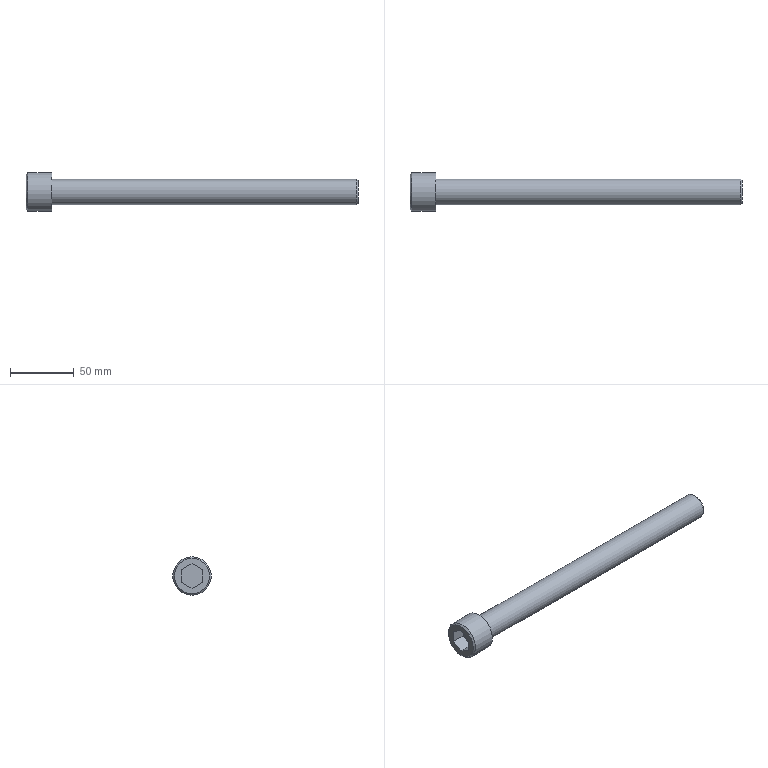Part | STEP file | solid 144 | 1 solid | 14 faces | box 260 x 30 x 30 mm | volume 86664 mm3 | plane 10 | cone 2 | cylinder 2 | commonest cylinder face diameters 20 x1 30 x1